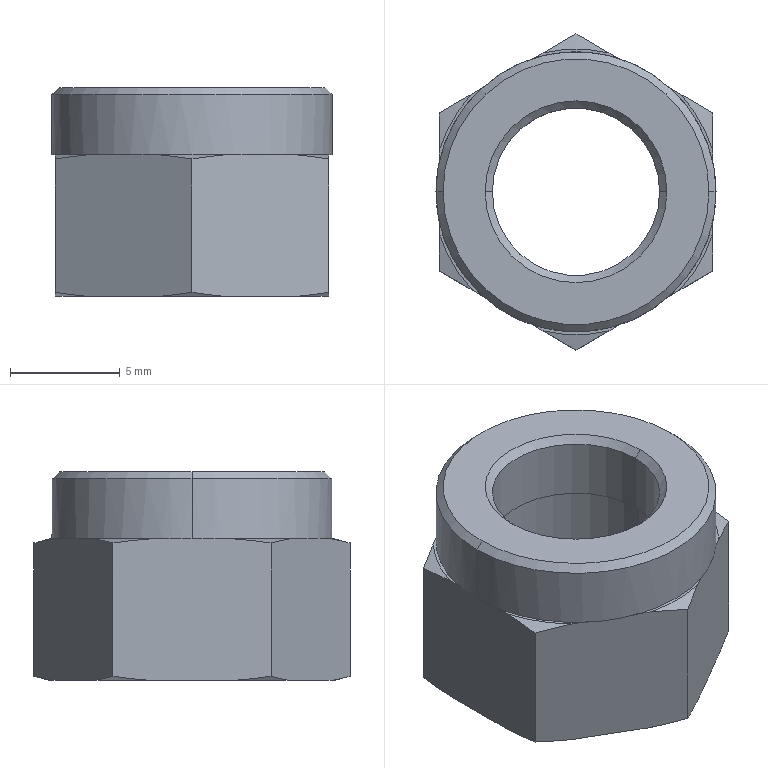Part | SolidWorks | features Cut 3, Boss 1, Chamfer 1, Extrusion 1 | 1 solid | 43 faces | box 12.74 x 14.38 x 9.5 mm | volume 787.765 mm3 | plane 21 | cone 16 | cylinder 6 | commonest cylinder face diameters 7.619 x2 8 x2 12.74 x2
STEP:
#1=CARTESIAN_POINT('',(-3.81,0.,9.175));
#2=VERTEX_POINT('',#1);
#3=CARTESIAN_POINT('',(3.81,0.,9.175));
#4=VERTEX_POINT('',#3);
#5=CARTESIAN_POINT('',(0.,0.,9.175));
#6=DIRECTION('',(0.,0.,1.));
#7=DIRECTION('',(1.,0.,0.));
#8=AXIS2_PLACEMENT_3D('',#5,#6,#7);
#9=CIRCLE('',#8,3.81);
#10=EDGE_CURVE('',#2,#4,#9,.T.);
#11=ORIENTED_EDGE('',*,*,#10,.F.);
#12=CARTESIAN_POINT('',(-4.135,0.,9.5));
#13=VERTEX_POINT('',#12);
#14=CARTESIAN_POINT('',(-3.81,0.,9.175));
#15=DIRECTION('',(-0.7071,0.,0.7071));
#16=VECTOR('',#15,1000.);
#17=LINE('',#14,#16);
#18=EDGE_CURVE('',#2,#13,#17,.T.);
#19=ORIENTED_EDGE('',*,*,#18,.T.);
#20=CARTESIAN_POINT('',(4.135,0.,9.5));
#21=VERTEX_POINT('',#20);
#22=CARTESIAN_POINT('',(0.,0.,9.5));
#23=DIRECTION('',(0.,0.,-1.));
#24=DIRECTION('',(1.,0.,0.));
#25=AXIS2_PLACEMENT_3D('',#22,#23,#24);
#26=CIRCLE('',#25,4.135);
#27=EDGE_CURVE('',#21,#13,#26,.T.);
#28=ORIENTED_EDGE('',*,*,#27,.F.);
#29=CARTESIAN_POINT('',(3.81,0.,9.175));
#30=DIRECTION('',(0.7071,0.,0.7071));
#31=VECTOR('',#30,1000.);
#32=LINE('',#29,#31);
#33=EDGE_CURVE('',#4,#21,#32,.T.);
#34=ORIENTED_EDGE('',*,*,#33,.F.);
#35=EDGE_LOOP('',(#11,#19,#28,#34));
#36=FACE_OUTER_BOUND('',#35,.T.);
#37=CARTESIAN_POINT('',(0.,0.,9.175));
#38=DIRECTION('',(0.,0.,1.));
#39=DIRECTION('',(1.,0.,0.));
#40=AXIS2_PLACEMENT_3D('',#37,#38,#39);
#41=CONICAL_SURFACE('',#40,3.81,0.7854);
#42=ADVANCED_FACE('',(#36),#41,.F.);
#43=CARTESIAN_POINT('',(6.045,0.,9.5));
#44=VERTEX_POINT('',#43);
#45=CARTESIAN_POINT('',(-6.045,0.,9.5));
#46=VERTEX_POINT('',#45);
#47=CARTESIAN_POINT('',(0.,0.,9.5));
#48=DIRECTION('',(0.,0.,1.));
#49=DIRECTION('',(1.,0.,0.));
#50=AXIS2_PLACEMENT_3D('',#47,#48,#49);
#51=CIRCLE('',#50,6.045);
#52=EDGE_CURVE('',#44,#46,#51,.T.);
#53=ORIENTED_EDGE('',*,*,#52,.F.);
#54=CARTESIAN_POINT('',(6.37,0.,9.175));
#55=VERTEX_POINT('',#54);
#56=CARTESIAN_POINT('',(6.045,0.,9.5));
#57=DIRECTION('',(0.7071,0.,-0.7071));
#58=VECTOR('',#57,1000.);
#59=LINE('',#56,#58);
#60=EDGE_CURVE('',#44,#55,#59,.T.);
#61=ORIENTED_EDGE('',*,*,#60,.T.);
#62=CARTESIAN_POINT('',(-6.37,0.,9.175));
#63=VERTEX_POINT('',#62);
#64=CARTESIAN_POINT('',(0.,0.,9.175));
#65=DIRECTION('',(0.,0.,-1.));
#66=DIRECTION('',(1.,0.,0.));
#67=AXIS2_PLACEMENT_3D('',#64,#65,#66);
#68=CIRCLE('',#67,6.37);
#69=EDGE_CURVE('',#63,#55,#68,.T.);
#70=ORIENTED_EDGE('',*,*,#69,.F.);
#71=CARTESIAN_POINT('',(-6.045,0.,9.5));
#72=DIRECTION('',(-0.7071,0.,-0.7071));
#73=VECTOR('',#72,1000.);
#74=LINE('',#71,#73);
#75=EDGE_CURVE('',#46,#63,#74,.T.);
#76=ORIENTED_EDGE('',*,*,#75,.F.);
#77=EDGE_LOOP('',(#53,#61,#70,#76));
#78=FACE_OUTER_BOUND('',#77,.T.);
#79=CARTESIAN_POINT('',(0.,0.,9.5));
#80=DIRECTION('',(0.,0.,-1.));
#81=DIRECTION('',(-1.,0.,0.));
#82=AXIS2_PLACEMENT_3D('',#79,#80,#81);
#83=CONICAL_SURFACE('',#82,6.045,0.7854);
#84=ADVANCED_FACE('',(#78),#83,.T.);
#85=CARTESIAN_POINT('',(-3.81,0.,6.44));
#86=VERTEX_POINT('',#85);
#87=CARTESIAN_POINT('',(3.81,0.,6.44));
#88=VERTEX_POINT('',#87);
#89=CARTESIAN_POINT('',(0.,0.,6.44));
#90=DIRECTION('',(0.,0.,1.));
#91=DIRECTION('',(1.,0.,0.));
#92=AXIS2_PLACEMENT_3D('',#89,#90,#91);
#93=CIRCLE('',#92,3.81);
#94=EDGE_CURVE('',#86,#88,#93,.T.);
#95=ORIENTED_EDGE('',*,*,#94,.F.);
#96=CARTESIAN_POINT('',(-3.81,0.,0.));
#97=DIRECTION('',(0.,0.,1.));
#98=VECTOR('',#97,1000.);
#99=LINE('',#96,#98);
#100=EDGE_CURVE('',#86,#2,#99,.T.);
#101=ORIENTED_EDGE('',*,*,#100,.T.);
#102=ORIENTED_EDGE('',*,*,#10,.T.);
#103=CARTESIAN_POINT('',(3.81,0.,0.));
#104=DIRECTION('',(0.,0.,1.));
#105=VECTOR('',#104,1000.);
#106=LINE('',#103,#105);
#107=EDGE_CURVE('',#88,#4,#106,.T.);
#108=ORIENTED_EDGE('',*,*,#107,.F.);
#109=EDGE_LOOP('',(#95,#101,#102,#108));
#110=FACE_OUTER_BOUND('',#109,.T.);
#111=CARTESIAN_POINT('',(0.,0.,0.));
#112=DIRECTION('',(0.,0.,1.));
#113=DIRECTION('',(1.,0.,0.));
#114=AXIS2_PLACEMENT_3D('',#111,#112,#113);
#115=CYLINDRICAL_SURFACE('',#114,3.81);
#116=ADVANCED_FACE('',(#110),#115,.F.);
#117=ORIENTED_EDGE('',*,*,#69,.T.);
#118=CARTESIAN_POINT('',(6.37,0.,6.44));
#119=VERTEX_POINT('',#118);
#120=CARTESIAN_POINT('',(6.37,0.,9.5));
#121=DIRECTION('',(0.,0.,-1.));
#122=VECTOR('',#121,1000.);
#123=LINE('',#120,#122);
#124=EDGE_CURVE('',#55,#119,#123,.T.);
#125=ORIENTED_EDGE('',*,*,#124,.T.);
#126=CARTESIAN_POINT('',(6.227,1.343,6.44));
#127=VERTEX_POINT('',#126);
#128=CARTESIAN_POINT('',(0.,0.,6.44));
#129=DIRECTION('',(0.,0.,1.));
#130=DIRECTION('',(1.,0.,0.));
#131=AXIS2_PLACEMENT_3D('',#128,#129,#130);
#132=CIRCLE('',#131,6.37);
#133=EDGE_CURVE('',#119,#127,#132,.T.);
#134=ORIENTED_EDGE('',*,*,#133,.T.);
#135=CARTESIAN_POINT('',(4.277,4.721,6.44));
#136=VERTEX_POINT('',#135);
#137=CARTESIAN_POINT('',(0.,0.,6.44));
#138=DIRECTION('',(0.,0.,1.));
#139=DIRECTION('',(1.,0.,0.));
#140=AXIS2_PLACEMENT_3D('',#137,#138,#139);
#141=CIRCLE('',#140,6.37);
#142=EDGE_CURVE('',#127,#136,#141,.T.);
#143=ORIENTED_EDGE('',*,*,#142,.T.);
#144=CARTESIAN_POINT('',(1.95,6.064,6.44));
#145=VERTEX_POINT('',#144);
#146=CARTESIAN_POINT('',(0.,0.,6.44));
#147=DIRECTION('',(0.,0.,1.));
#148=DIRECTION('',(1.,0.,0.));
#149=AXIS2_PLACEMENT_3D('',#146,#147,#148);
#150=CIRCLE('',#149,6.37);
#151=EDGE_CURVE('',#136,#145,#150,.T.);
#152=ORIENTED_EDGE('',*,*,#151,.T.);
#153=CARTESIAN_POINT('',(-1.95,6.064,6.44));
#154=VERTEX_POINT('',#153);
#155=CARTESIAN_POINT('',(0.,0.,6.44));
#156=DIRECTION('',(0.,0.,1.));
#157=DIRECTION('',(1.,0.,0.));
#158=AXIS2_PLACEMENT_3D('',#155,#156,#157);
#159=CIRCLE('',#158,6.37);
#160=EDGE_CURVE('',#145,#154,#159,.T.);
#161=ORIENTED_EDGE('',*,*,#160,.T.);
#162=CARTESIAN_POINT('',(-4.277,4.721,6.44));
#163=VERTEX_POINT('',#162);
#164=CARTESIAN_POINT('',(0.,0.,6.44));
#165=DIRECTION('',(0.,0.,1.));
#166=DIRECTION('',(1.,0.,0.));
#167=AXIS2_PLACEMENT_3D('',#164,#165,#166);
#168=CIRCLE('',#167,6.37);
#169=EDGE_CURVE('',#154,#163,#168,.T.);
#170=ORIENTED_EDGE('',*,*,#169,.T.);
#171=CARTESIAN_POINT('',(-6.227,1.343,6.44));
#172=VERTEX_POINT('',#171);
#173=CARTESIAN_POINT('',(0.,0.,6.44));
#174=DIRECTION('',(0.,0.,1.));
#175=DIRECTION('',(1.,0.,0.));
#176=AXIS2_PLACEMENT_3D('',#173,#174,#175);
#177=CIRCLE('',#176,6.37);
#178=EDGE_CURVE('',#163,#172,#177,.T.);
#179=ORIENTED_EDGE('',*,*,#178,.T.);
#180=CARTESIAN_POINT('',(-6.37,0.,6.44));
#181=VERTEX_POINT('',#180);
#182=CARTESIAN_POINT('',(0.,0.,6.44));
#183=DIRECTION('',(0.,0.,1.));
#184=DIRECTION('',(1.,0.,0.));
#185=AXIS2_PLACEMENT_3D('',#182,#183,#184);
#186=CIRCLE('',#185,6.37);
#187=EDGE_CURVE('',#172,#181,#186,.T.);
#188=ORIENTED_EDGE('',*,*,#187,.T.);
#189=CARTESIAN_POINT('',(-6.37,0.,9.5));
#190=DIRECTION('',(0.,0.,-1.));
#191=VECTOR('',#190,1000.);
#192=LINE('',#189,#191);
#193=EDGE_CURVE('',#63,#181,#192,.T.);
#194=ORIENTED_EDGE('',*,*,#193,.F.);
#195=EDGE_LOOP('',(#117,#125,#134,#143,#152,#161,#170,#179,#188,#194));
#196=FACE_OUTER_BOUND('',#195,.T.);
#197=CARTESIAN_POINT('',(0.,0.,9.5));
#198=DIRECTION('',(0.,0.,-1.));
#199=DIRECTION('',(-1.,0.,0.));
#200=AXIS2_PLACEMENT_3D('',#197,#198,#199);
#201=CYLINDRICAL_SURFACE('',#200,6.37);
#202=ADVANCED_FACE('',(#196),#201,.T.);
#203=CARTESIAN_POINT('',(-4.,0.,6.44));
#204=VERTEX_POINT('',#203);
#205=CARTESIAN_POINT('',(4.,0.,6.44));
#206=VERTEX_POINT('',#205);
#207=CARTESIAN_POINT('',(0.,0.,6.44));
#208=DIRECTION('',(0.,0.,1.));
#209=DIRECTION('',(1.,0.,0.));
#210=AXIS2_PLACEMENT_3D('',#207,#208,#209);
#211=CIRCLE('',#210,4.);
#212=EDGE_CURVE('',#204,#206,#211,.T.);
#213=ORIENTED_EDGE('',*,*,#212,.T.);
#214=CARTESIAN_POINT('',(4.,0.,0.));
#215=VERTEX_POINT('',#214);
#216=CARTESIAN_POINT('',(4.,0.,6.44));
#217=DIRECTION('',(0.,0.,-1.));
#218=VECTOR('',#217,1000.);
#219=LINE('',#216,#218);
#220=EDGE_CURVE('',#206,#215,#219,.T.);
#221=ORIENTED_EDGE('',*,*,#220,.T.);
#222=CARTESIAN_POINT('',(-4.,0.,0.));
#223=VERTEX_POINT('',#222);
#224=CARTESIAN_POINT('',(0.,0.,0.));
#225=DIRECTION('',(0.,0.,1.));
#226=DIRECTION('',(1.,0.,0.));
#227=AXIS2_PLACEMENT_3D('',#224,#225,#226);
#228=CIRCLE('',#227,4.);
#229=EDGE_CURVE('',#223,#215,#228,.T.);
#230=ORIENTED_EDGE('',*,*,#229,.F.);
#231=CARTESIAN_POINT('',(-4.,0.,6.44));
#232=DIRECTION('',(0.,0.,-1.));
#233=VECTOR('',#232,1000.);
#234=LINE('',#231,#233);
#235=EDGE_CURVE('',#204,#223,#234,.T.);
#236=ORIENTED_EDGE('',*,*,#235,.F.);
#237=EDGE_LOOP('',(#213,#221,#230,#236));
#238=FACE_OUTER_BOUND('',#237,.T.);
#239=CARTESIAN_POINT('',(0.,0.,6.44));
#240=DIRECTION('',(0.,0.,-1.));
#241=DIRECTION('',(-1.,0.,0.));
#242=AXIS2_PLACEMENT_3D('',#239,#240,#241);
#243=CYLINDRICAL_SURFACE('',#242,4.);
#244=ADVANCED_FACE('',(#238),#243,.F.);
#245=CARTESIAN_POINT('',(-6.227,-1.343,6.44));
#246=VERTEX_POINT('',#245);
#247=CARTESIAN_POINT('',(-4.277,-4.721,6.44));
#248=VERTEX_POINT('',#247);
#249=CARTESIAN_POINT('',(0.,0.,6.44));
#250=DIRECTION('',(0.,0.,1.));
#251=DIRECTION('',(1.,0.,0.));
#252=AXIS2_PLACEMENT_3D('',#249,#250,#251);
#253=CIRCLE('',#252,6.37);
#254=EDGE_CURVE('',#246,#248,#253,.T.);
#255=ORIENTED_EDGE('',*,*,#254,.F.);
#256=CARTESIAN_POINT('',(-6.227,-1.865,6.44));
#257=VERTEX_POINT('',#256);
#258=CARTESIAN_POINT('',(-6.227,3.595,6.44));
#259=DIRECTION('',(0.,-1.,0.));
#260=VECTOR('',#259,1000.);
#261=LINE('',#258,#260);
#262=EDGE_CURVE('',#246,#257,#261,.T.);
#263=ORIENTED_EDGE('',*,*,#262,.T.);
#264=CARTESIAN_POINT('',(-4.728,-4.46,6.44));
#265=VERTEX_POINT('',#264);
#266=CARTESIAN_POINT('',(0.,0.,6.44));
#267=DIRECTION('',(0.,0.,1.));
#268=DIRECTION('',(1.,0.,0.));
#269=AXIS2_PLACEMENT_3D('',#266,#267,#268);
#270=CIRCLE('',#269,6.5);
#271=EDGE_CURVE('',#257,#265,#270,.T.);
#272=ORIENTED_EDGE('',*,*,#271,.T.);
#273=CARTESIAN_POINT('',(-6.227,-3.595,6.44));
#274=DIRECTION('',(0.866,-0.5,0.));
#275=VECTOR('',#274,1000.);
#276=LINE('',#273,#275);
#277=EDGE_CURVE('',#265,#248,#276,.T.);
#278=ORIENTED_EDGE('',*,*,#277,.T.);
#279=EDGE_LOOP('',(#255,#263,#272,#278));
#280=FACE_OUTER_BOUND('',#279,.T.);
#281=CARTESIAN_POINT('',(6.227,3.595,6.44));
#282=DIRECTION('',(0.,0.,-1.));
#283=DIRECTION('',(-1.,0.,0.));
#284=AXIS2_PLACEMENT_3D('',#281,#282,#283);
#285=PLANE('',#284);
#286=ADVANCED_FACE('',(#280),#285,.F.);
#287=CARTESIAN_POINT('',(-1.95,-6.064,6.44));
#288=VERTEX_POINT('',#287);
#289=CARTESIAN_POINT('',(1.95,-6.064,6.44));
#290=VERTEX_POINT('',#289);
#291=CARTESIAN_POINT('',(0.,0.,6.44));
#292=DIRECTION('',(0.,0.,1.));
#293=DIRECTION('',(1.,0.,0.));
#294=AXIS2_PLACEMENT_3D('',#291,#292,#293);
#295=CIRCLE('',#294,6.37);
#296=EDGE_CURVE('',#288,#290,#295,.T.);
#297=ORIENTED_EDGE('',*,*,#296,.F.);
#298=CARTESIAN_POINT('',(-1.498,-6.325,6.44));
#299=VERTEX_POINT('',#298);
#300=CARTESIAN_POINT('',(-6.227,-3.595,6.44));
#301=DIRECTION('',(0.866,-0.5,0.));
#302=VECTOR('',#301,1000.);
#303=LINE('',#300,#302);
#304=EDGE_CURVE('',#288,#299,#303,.T.);
#305=ORIENTED_EDGE('',*,*,#304,.T.);
#306=CARTESIAN_POINT('',(1.498,-6.325,6.44));
#307=VERTEX_POINT('',#306);
#308=CARTESIAN_POINT('',(0.,0.,6.44));
#309=DIRECTION('',(0.,0.,1.));
#310=DIRECTION('',(1.,0.,0.));
#311=AXIS2_PLACEMENT_3D('',#308,#309,#310);
#312=CIRCLE('',#311,6.5);
#313=EDGE_CURVE('',#299,#307,#312,.T.);
#314=ORIENTED_EDGE('',*,*,#313,.T.);
#315=CARTESIAN_POINT('',(0.,-7.19,6.44));
#316=DIRECTION('',(0.866,0.5,0.));
#317=VECTOR('',#316,1000.);
#318=LINE('',#315,#317);
#319=EDGE_CURVE('',#307,#290,#318,.T.);
#320=ORIENTED_EDGE('',*,*,#319,.T.);
#321=EDGE_LOOP('',(#297,#305,#314,#320));
#322=FACE_OUTER_BOUND('',#321,.T.);
#323=CARTESIAN_POINT('',(6.227,3.595,6.44));
#324=DIRECTION('',(0.,0.,-1.));
#325=DIRECTION('',(-1.,0.,0.));
#326=AXIS2_PLACEMENT_3D('',#323,#324,#325);
#327=PLANE('',#326);
#328=ADVANCED_FACE('',(#322),#327,.F.);
#329=CARTESIAN_POINT('',(4.277,-4.721,6.44));
#330=VERTEX_POINT('',#329);
#331=CARTESIAN_POINT('',(6.227,-1.343,6.44));
#332=VERTEX_POINT('',#331);
#333=CARTESIAN_POINT('',(0.,0.,6.44));
#334=DIRECTION('',(0.,0.,1.));
#335=DIRECTION('',(1.,0.,0.));
#336=AXIS2_PLACEMENT_3D('',#333,#334,#335);
#337=CIRCLE('',#336,6.37);
#338=EDGE_CURVE('',#330,#332,#337,.T.);
#339=ORIENTED_EDGE('',*,*,#338,.F.);
#340=CARTESIAN_POINT('',(4.728,-4.46,6.44));
#341=VERTEX_POINT('',#340);
#342=CARTESIAN_POINT('',(0.,-7.19,6.44));
#343=DIRECTION('',(0.866,0.5,0.));
#344=VECTOR('',#343,1000.);
#345=LINE('',#342,#344);
#346=EDGE_CURVE('',#330,#341,#345,.T.);
#347=ORIENTED_EDGE('',*,*,#346,.T.);
#348=CARTESIAN_POINT('',(6.227,-1.865,6.44));
#349=VERTEX_POINT('',#348);
#350=CARTESIAN_POINT('',(0.,0.,6.44));
#351=DIRECTION('',(0.,0.,1.));
#352=DIRECTION('',(1.,0.,0.));
#353=AXIS2_PLACEMENT_3D('',#350,#351,#352);
#354=CIRCLE('',#353,6.5);
#355=EDGE_CURVE('',#341,#349,#354,.T.);
#356=ORIENTED_EDGE('',*,*,#355,.T.);
#357=CARTESIAN_POINT('',(6.227,-3.595,6.44));
#358=DIRECTION('',(0.,1.,0.));
#359=VECTOR('',#358,1000.);
#360=LINE('',#357,#359);
#361=EDGE_CURVE('',#349,#332,#360,.T.);
#362=ORIENTED_EDGE('',*,*,#361,.T.);
#363=EDGE_LOOP('',(#339,#347,#356,#362));
#364=FACE_OUTER_BOUND('',#363,.T.);
#365=CARTESIAN_POINT('',(6.227,3.595,6.44));
#366=DIRECTION('',(0.,0.,-1.));
#367=DIRECTION('',(-1.,0.,0.));
#368=AXIS2_PLACEMENT_3D('',#365,#366,#367);
#369=PLANE('',#368);
#370=ADVANCED_FACE('',(#364),#369,.F.);
#371=ORIENTED_EDGE('',*,*,#142,.F.);
#372=CARTESIAN_POINT('',(6.227,1.865,6.44));
#373=VERTEX_POINT('',#372);
#374=CARTESIAN_POINT('',(6.227,-3.595,6.44));
#375=DIRECTION('',(0.,1.,0.));
#376=VECTOR('',#375,1000.);
#377=LINE('',#374,#376);
#378=EDGE_CURVE('',#127,#373,#377,.T.);
#379=ORIENTED_EDGE('',*,*,#378,.T.);
#380=CARTESIAN_POINT('',(4.728,4.46,6.44));
#381=VERTEX_POINT('',#380);
#382=CARTESIAN_POINT('',(0.,0.,6.44));
#383=DIRECTION('',(0.,0.,1.));
#384=DIRECTION('',(1.,0.,0.));
#385=AXIS2_PLACEMENT_3D('',#382,#383,#384);
#386=CIRCLE('',#385,6.5);
#387=EDGE_CURVE('',#373,#381,#386,.T.);
#388=ORIENTED_EDGE('',*,*,#387,.T.);
#389=CARTESIAN_POINT('',(6.227,3.595,6.44));
#390=DIRECTION('',(-0.866,0.5,0.));
#391=VECTOR('',#390,1000.);
#392=LINE('',#389,#391);
#393=EDGE_CURVE('',#381,#136,#392,.T.);
#394=ORIENTED_EDGE('',*,*,#393,.T.);
#395=EDGE_LOOP('',(#371,#379,#388,#394));
#396=FACE_OUTER_BOUND('',#395,.T.);
#397=CARTESIAN_POINT('',(6.227,3.595,6.44));
#398=DIRECTION('',(0.,0.,-1.));
#399=DIRECTION('',(-1.,0.,0.));
#400=AXIS2_PLACEMENT_3D('',#397,#398,#399);
#401=PLANE('',#400);
#402=ADVANCED_FACE('',(#396),#401,.F.);
#403=ORIENTED_EDGE('',*,*,#160,.F.);
#404=CARTESIAN_POINT('',(1.498,6.325,6.44));
#405=VERTEX_POINT('',#404);
#406=CARTESIAN_POINT('',(6.227,3.595,6.44));
#407=DIRECTION('',(-0.866,0.5,0.));
#408=VECTOR('',#407,1000.);
#409=LINE('',#406,#408);
#410=EDGE_CURVE('',#145,#405,#409,.T.);
#411=ORIENTED_EDGE('',*,*,#410,.T.);
#412=CARTESIAN_POINT('',(-1.498,6.325,6.44));
#413=VERTEX_POINT('',#412);
#414=CARTESIAN_POINT('',(0.,0.,6.44));
#415=DIRECTION('',(0.,0.,1.));
#416=DIRECTION('',(1.,0.,0.));
#417=AXIS2_PLACEMENT_3D('',#414,#415,#416);
#418=CIRCLE('',#417,6.5);
#419=EDGE_CURVE('',#405,#413,#418,.T.);
#420=ORIENTED_EDGE('',*,*,#419,.T.);
#421=CARTESIAN_POINT('',(0.,7.19,6.44));
#422=DIRECTION('',(-0.866,-0.5,0.));
#423=VECTOR('',#422,1000.);
#424=LINE('',#421,#423);
#425=EDGE_CURVE('',#413,#154,#424,.T.);
#426=ORIENTED_EDGE('',*,*,#425,.T.);
#427=EDGE_LOOP('',(#403,#411,#420,#426));
#428=FACE_OUTER_BOUND('',#427,.T.);
#429=CARTESIAN_POINT('',(6.227,3.595,6.44));
#430=DIRECTION('',(0.,0.,-1.));
#431=DIRECTION('',(-1.,0.,0.));
#432=AXIS2_PLACEMENT_3D('',#429,#430,#431);
#433=PLANE('',#432);
#434=ADVANCED_FACE('',(#428),#433,.F.);
#435=ORIENTED_EDGE('',*,*,#178,.F.);
#436=CARTESIAN_POINT('',(-4.728,4.46,6.44));
#437=VERTEX_POINT('',#436);
#438=CARTESIAN_POINT('',(0.,7.19,6.44));
#439=DIRECTION('',(-0.866,-0.5,0.));
#440=VECTOR('',#439,1000.);
#441=LINE('',#438,#440);
#442=EDGE_CURVE('',#163,#437,#441,.T.);
#443=ORIENTED_EDGE('',*,*,#442,.T.);
#444=CARTESIAN_POINT('',(-6.227,1.865,6.44));
#445=VERTEX_POINT('',#444);
#446=CARTESIAN_POINT('',(0.,0.,6.44));
#447=DIRECTION('',(0.,0.,1.));
#448=DIRECTION('',(1.,0.,0.));
#449=AXIS2_PLACEMENT_3D('',#446,#447,#448);
#450=CIRCLE('',#449,6.5);
#451=EDGE_CURVE('',#437,#445,#450,.T.);
#452=ORIENTED_EDGE('',*,*,#451,.T.);
#453=CARTESIAN_POINT('',(-6.227,3.595,6.44));
#454=DIRECTION('',(0.,-1.,0.));
#455=VECTOR('',#454,1000.);
#456=LINE('',#453,#455);
#457=EDGE_CURVE('',#445,#172,#456,.T.);
#458=ORIENTED_EDGE('',*,*,#457,.T.);
#459=EDGE_LOOP('',(#435,#443,#452,#458));
#460=FACE_OUTER_BOUND('',#459,.T.);
#461=CARTESIAN_POINT('',(6.227,3.595,6.44));
#462=DIRECTION('',(0.,0.,-1.));
#463=DIRECTION('',(-1.,0.,0.));
#464=AXIS2_PLACEMENT_3D('',#461,#462,#463);
#465=PLANE('',#464);
#466=ADVANCED_FACE('',(#460),#465,.F.);
#467=CARTESIAN_POINT('',(0.,7.19,0.1849));
#468=VERTEX_POINT('',#467);
#469=CARTESIAN_POINT('',(1.498,6.325,0.));
#470=VERTEX_POINT('',#469);
#471=CARTESIAN_POINT('',(0.,7.19,0.1849));
#472=CARTESIAN_POINT('',(0.4978,6.903,0.1079));
#473=CARTESIAN_POINT('',(0.9971,6.614,0.04449));
#474=CARTESIAN_POINT('',(1.498,6.325,0.));
#475=B_SPLINE_CURVE_WITH_KNOTS('',3,(#471,#472,#473,#474),.UNSPECIFIED.,.F.,.F.,(4,4),(0.006757,0.008497),.UNSPECIFIED.);
#476=EDGE_CURVE('',#468,#470,#475,.T.);
#477=ORIENTED_EDGE('',*,*,#476,.F.);
#478=CARTESIAN_POINT('',(0.,7.19,6.255));
#479=VERTEX_POINT('',#478);
#480=CARTESIAN_POINT('',(0.,7.19,6.44));
#481=DIRECTION('',(0.,0.,-1.));
#482=VECTOR('',#481,1000.);
#483=LINE('',#480,#482);
#484=EDGE_CURVE('',#479,#468,#483,.T.);
#485=ORIENTED_EDGE('',*,*,#484,.F.);
#486=CARTESIAN_POINT('',(1.498,6.325,6.44));
#487=CARTESIAN_POINT('',(0.9966,6.615,6.395));
#488=CARTESIAN_POINT('',(0.4971,6.903,6.332));
#489=CARTESIAN_POINT('',(0.,7.19,6.255));
#490=B_SPLINE_CURVE_WITH_KNOTS('',3,(#486,#487,#488,#489),.UNSPECIFIED.,.F.,.F.,(4,4),(0.0122,0.01391),.UNSPECIFIED.);
#491=EDGE_CURVE('',#405,#479,#490,.T.);
#492=ORIENTED_EDGE('',*,*,#491,.F.);
#493=ORIENTED_EDGE('',*,*,#410,.F.);
#494=CARTESIAN_POINT('',(6.227,3.595,6.44));
#495=DIRECTION('',(-0.866,0.5,0.));
#496=VECTOR('',#495,1000.);
#497=LINE('',#494,#496);
#498=EDGE_CURVE('',#136,#145,#497,.T.);
#499=ORIENTED_EDGE('',*,*,#498,.F.);
#500=ORIENTED_EDGE('',*,*,#393,.F.);
#501=CARTESIAN_POINT('',(6.227,3.595,6.255));
#502=VERTEX_POINT('',#501);
#503=CARTESIAN_POINT('',(6.227,3.595,6.255));
#504=CARTESIAN_POINT('',(5.729,3.882,6.332));
#505=CARTESIAN_POINT('',(5.23,4.171,6.396));
#506=CARTESIAN_POINT('',(4.728,4.46,6.44));
#507=B_SPLINE_CURVE_WITH_KNOTS('',3,(#503,#504,#505,#506),.UNSPECIFIED.,.F.,.F.,(4,4),(0.006757,0.008497),.UNSPECIFIED.);
#508=EDGE_CURVE('',#502,#381,#507,.T.);
#509=ORIENTED_EDGE('',*,*,#508,.F.);
#510=CARTESIAN_POINT('',(6.227,3.595,0.1849));
#511=VERTEX_POINT('',#510);
#512=CARTESIAN_POINT('',(6.227,3.595,6.44));
#513=DIRECTION('',(0.,0.,-1.));
#514=VECTOR('',#513,1000.);
#515=LINE('',#512,#514);
#516=EDGE_CURVE('',#502,#511,#515,.T.);
#517=ORIENTED_EDGE('',*,*,#516,.T.);
#518=CARTESIAN_POINT('',(4.728,4.46,0.));
#519=VERTEX_POINT('',#518);
#520=CARTESIAN_POINT('',(4.728,4.46,0.));
#521=CARTESIAN_POINT('',(5.23,4.17,0.04453));
#522=CARTESIAN_POINT('',(5.73,3.882,0.108));
#523=CARTESIAN_POINT('',(6.227,3.595,0.1849));
#524=B_SPLINE_CURVE_WITH_KNOTS('',3,(#520,#521,#522,#523),.UNSPECIFIED.,.F.,.F.,(4,4),(0.0122,0.01391),.UNSPECIFIED.);
#525=EDGE_CURVE('',#519,#511,#524,.T.);
#526=ORIENTED_EDGE('',*,*,#525,.F.);
#527=CARTESIAN_POINT('',(6.227,3.595,0.));
#528=DIRECTION('',(-0.866,0.5,0.));
#529=VECTOR('',#528,1000.);
#530=LINE('',#527,#529);
#531=EDGE_CURVE('',#519,#470,#530,.T.);
#532=ORIENTED_EDGE('',*,*,#531,.T.);
#533=EDGE_LOOP('',(#477,#485,#492,#493,#499,#500,#509,#517,#526,#532));
#534=FACE_OUTER_BOUND('',#533,.T.);
#535=CARTESIAN_POINT('',(6.227,3.595,6.44));
#536=DIRECTION('',(-0.5,-0.866,0.));
#537=DIRECTION('',(0.866,-0.5,0.));
#538=AXIS2_PLACEMENT_3D('',#535,#536,#537);
#539=PLANE('',#538);
#540=ADVANCED_FACE('',(#534),#539,.F.);
#541=CARTESIAN_POINT('',(-6.227,3.595,0.1849));
#542=VERTEX_POINT('',#541);
#543=CARTESIAN_POINT('',(-4.728,4.46,0.));
#544=VERTEX_POINT('',#543);
#545=CARTESIAN_POINT('',(-6.227,3.595,0.1849));
#546=CARTESIAN_POINT('',(-5.729,3.882,0.1079));
#547=CARTESIAN_POINT('',(-5.23,4.171,0.04449));
#548=CARTESIAN_POINT('',(-4.728,4.46,0.));
#549=B_SPLINE_CURVE_WITH_KNOTS('',3,(#545,#546,#547,#548),.UNSPECIFIED.,.F.,.F.,(4,4),(0.006757,0.008497),.UNSPECIFIED.);
#550=EDGE_CURVE('',#542,#544,#549,.T.);
#551=ORIENTED_EDGE('',*,*,#550,.F.);
#552=CARTESIAN_POINT('',(-6.227,3.595,6.255));
#553=VERTEX_POINT('',#552);
#554=CARTESIAN_POINT('',(-6.227,3.595,6.44));
#555=DIRECTION('',(0.,0.,-1.));
#556=VECTOR('',#555,1000.);
#557=LINE('',#554,#556);
#558=EDGE_CURVE('',#553,#542,#557,.T.);
#559=ORIENTED_EDGE('',*,*,#558,.F.);
#560=CARTESIAN_POINT('',(-4.728,4.46,6.44));
#561=CARTESIAN_POINT('',(-5.23,4.17,6.395));
#562=CARTESIAN_POINT('',(-5.73,3.882,6.332));
#563=CARTESIAN_POINT('',(-6.227,3.595,6.255));
#564=B_SPLINE_CURVE_WITH_KNOTS('',3,(#560,#561,#562,#563),.UNSPECIFIED.,.F.,.F.,(4,4),(0.0122,0.01391),.UNSPECIFIED.);
#565=EDGE_CURVE('',#437,#553,#564,.T.);
#566=ORIENTED_EDGE('',*,*,#565,.F.);
#567=ORIENTED_EDGE('',*,*,#442,.F.);
#568=CARTESIAN_POINT('',(0.,7.19,6.44));
#569=DIRECTION('',(-0.866,-0.5,0.));
#570=VECTOR('',#569,1000.);
#571=LINE('',#568,#570);
#572=EDGE_CURVE('',#154,#163,#571,.T.);
#573=ORIENTED_EDGE('',*,*,#572,.F.);
#574=ORIENTED_EDGE('',*,*,#425,.F.);
#575=CARTESIAN_POINT('',(0.,7.19,6.255));
#576=CARTESIAN_POINT('',(-0.4978,6.903,6.332));
#577=CARTESIAN_POINT('',(-0.9971,6.614,6.396));
#578=CARTESIAN_POINT('',(-1.498,6.325,6.44));
#579=B_SPLINE_CURVE_WITH_KNOTS('',3,(#575,#576,#577,#578),.UNSPECIFIED.,.F.,.F.,(4,4),(0.006757,0.008497),.UNSPECIFIED.);
#580=EDGE_CURVE('',#479,#413,#579,.T.);
#581=ORIENTED_EDGE('',*,*,#580,.F.);
#582=ORIENTED_EDGE('',*,*,#484,.T.);
#583=CARTESIAN_POINT('',(-1.498,6.325,0.));
#584=VERTEX_POINT('',#583);
#585=CARTESIAN_POINT('',(-1.498,6.325,0.));
#586=CARTESIAN_POINT('',(-0.9966,6.615,0.04453));
#587=CARTESIAN_POINT('',(-0.4971,6.903,0.108));
#588=CARTESIAN_POINT('',(0.,7.19,0.1849));
#589=B_SPLINE_CURVE_WITH_KNOTS('',3,(#585,#586,#587,#588),.UNSPECIFIED.,.F.,.F.,(4,4),(0.0122,0.01391),.UNSPECIFIED.);
#590=EDGE_CURVE('',#584,#468,#589,.T.);
#591=ORIENTED_EDGE('',*,*,#590,.F.);
#592=CARTESIAN_POINT('',(0.,7.19,0.));
#593=DIRECTION('',(-0.866,-0.5,0.));
#594=VECTOR('',#593,1000.);
#595=LINE('',#592,#594);
#596=EDGE_CURVE('',#584,#544,#595,.T.);
#597=ORIENTED_EDGE('',*,*,#596,.T.);
#598=EDGE_LOOP('',(#551,#559,#566,#567,#573,#574,#581,#582,#591,#597));
#599=FACE_OUTER_BOUND('',#598,.T.);
#600=CARTESIAN_POINT('',(0.,7.19,6.44));
#601=DIRECTION('',(0.5,-0.866,0.));
#602=DIRECTION('',(0.866,0.5,0.));
#603=AXIS2_PLACEMENT_3D('',#600,#601,#602);
#604=PLANE('',#603);
#605=ADVANCED_FACE('',(#599),#604,.F.);
#606=CARTESIAN_POINT('',(-6.227,-3.595,0.1849));
#607=VERTEX_POINT('',#606);
#608=CARTESIAN_POINT('',(-6.227,-1.865,0.));
#609=VERTEX_POINT('',#608);
#610=CARTESIAN_POINT('',(-6.227,-3.595,0.1849));
#611=CARTESIAN_POINT('',(-6.227,-3.02,0.1078));
#612=CARTESIAN_POINT('',(-6.227,-2.443,0.04448));
#613=CARTESIAN_POINT('',(-6.227,-1.865,0.));
#614=B_SPLINE_CURVE_WITH_KNOTS('',3,(#610,#611,#612,#613),.UNSPECIFIED.,.F.,.F.,(4,4),(0.005844,0.007584),.UNSPECIFIED.);
#615=EDGE_CURVE('',#607,#609,#614,.T.);
#616=ORIENTED_EDGE('',*,*,#615,.F.);
#617=CARTESIAN_POINT('',(-6.227,-3.595,6.255));
#618=VERTEX_POINT('',#617);
#619=CARTESIAN_POINT('',(-6.227,-3.595,6.44));
#620=DIRECTION('',(0.,0.,-1.));
#621=VECTOR('',#620,1000.);
#622=LINE('',#619,#621);
#623=EDGE_CURVE('',#618,#607,#622,.T.);
#624=ORIENTED_EDGE('',*,*,#623,.F.);
#625=CARTESIAN_POINT('',(-6.227,-1.865,6.44));
#626=CARTESIAN_POINT('',(-6.227,-2.443,6.396));
#627=CARTESIAN_POINT('',(-6.227,-3.021,6.332));
#628=CARTESIAN_POINT('',(-6.227,-3.595,6.255));
#629=B_SPLINE_CURVE_WITH_KNOTS('',3,(#625,#626,#627,#628),.UNSPECIFIED.,.F.,.F.,(4,4),(0.01129,0.013),.UNSPECIFIED.);
#630=EDGE_CURVE('',#257,#618,#629,.T.);
#631=ORIENTED_EDGE('',*,*,#630,.F.);
#632=ORIENTED_EDGE('',*,*,#262,.F.);
#633=CARTESIAN_POINT('',(-6.227,3.595,6.44));
#634=DIRECTION('',(0.,-1.,0.));
#635=VECTOR('',#634,1000.);
#636=LINE('',#633,#635);
#637=EDGE_CURVE('',#172,#246,#636,.T.);
#638=ORIENTED_EDGE('',*,*,#637,.F.);
#639=ORIENTED_EDGE('',*,*,#457,.F.);
#640=CARTESIAN_POINT('',(-6.227,3.595,6.255));
#641=CARTESIAN_POINT('',(-6.227,3.02,6.332));
#642=CARTESIAN_POINT('',(-6.227,2.443,6.396));
#643=CARTESIAN_POINT('',(-6.227,1.865,6.44));
#644=B_SPLINE_CURVE_WITH_KNOTS('',3,(#640,#641,#642,#643),.UNSPECIFIED.,.F.,.F.,(4,4),(0.005844,0.007584),.UNSPECIFIED.);
#645=EDGE_CURVE('',#553,#445,#644,.T.);
#646=ORIENTED_EDGE('',*,*,#645,.F.);
#647=ORIENTED_EDGE('',*,*,#558,.T.);
#648=CARTESIAN_POINT('',(-6.227,1.865,0.));
#649=VERTEX_POINT('',#648);
#650=CARTESIAN_POINT('',(-6.227,1.865,0.));
#651=CARTESIAN_POINT('',(-6.227,2.443,0.04447));
#652=CARTESIAN_POINT('',(-6.227,3.021,0.108));
#653=CARTESIAN_POINT('',(-6.227,3.595,0.1849));
#654=B_SPLINE_CURVE_WITH_KNOTS('',3,(#650,#651,#652,#653),.UNSPECIFIED.,.F.,.F.,(4,4),(0.01129,0.013),.UNSPECIFIED.);
#655=EDGE_CURVE('',#649,#542,#654,.T.);
#656=ORIENTED_EDGE('',*,*,#655,.F.);
#657=CARTESIAN_POINT('',(-6.227,3.595,0.));
#658=DIRECTION('',(0.,-1.,0.));
#659=VECTOR('',#658,1000.);
#660=LINE('',#657,#659);
#661=EDGE_CURVE('',#649,#609,#660,.T.);
#662=ORIENTED_EDGE('',*,*,#661,.T.);
#663=EDGE_LOOP('',(#616,#624,#631,#632,#638,#639,#646,#647,#656,#662));
#664=FACE_OUTER_BOUND('',#663,.T.);
#665=CARTESIAN_POINT('',(-6.227,3.595,6.44));
#666=DIRECTION('',(1.,0.,0.));
#667=DIRECTION('',(0.,0.,-1.));
#668=AXIS2_PLACEMENT_3D('',#665,#666,#667);
#669=PLANE('',#668);
#670=ADVANCED_FACE('',(#664),#669,.F.);
#671=CARTESIAN_POINT('',(0.,-7.19,0.1849));
#672=VERTEX_POINT('',#671);
#673=CARTESIAN_POINT('',(-1.498,-6.325,0.));
#674=VERTEX_POINT('',#673);
#675=CARTESIAN_POINT('',(0.,-7.19,0.1849));
#676=CARTESIAN_POINT('',(-0.4978,-6.903,0.1079));
#677=CARTESIAN_POINT('',(-0.9971,-6.614,0.04449));
#678=CARTESIAN_POINT('',(-1.498,-6.325,0.));
#679=B_SPLINE_CURVE_WITH_KNOTS('',3,(#675,#676,#677,#678),.UNSPECIFIED.,.F.,.F.,(4,4),(0.006757,0.008497),.UNSPECIFIED.);
#680=EDGE_CURVE('',#672,#674,#679,.T.);
#681=ORIENTED_EDGE('',*,*,#680,.F.);
#682=CARTESIAN_POINT('',(0.,-7.19,6.255));
#683=VERTEX_POINT('',#682);
#684=CARTESIAN_POINT('',(0.,-7.19,6.44));
#685=DIRECTION('',(0.,0.,-1.));
#686=VECTOR('',#685,1000.);
#687=LINE('',#684,#686);
#688=EDGE_CURVE('',#683,#672,#687,.T.);
#689=ORIENTED_EDGE('',*,*,#688,.F.);
#690=CARTESIAN_POINT('',(-1.498,-6.325,6.44));
#691=CARTESIAN_POINT('',(-0.9966,-6.615,6.395));
#692=CARTESIAN_POINT('',(-0.4971,-6.903,6.332));
#693=CARTESIAN_POINT('',(0.,-7.19,6.255));
#694=B_SPLINE_CURVE_WITH_KNOTS('',3,(#690,#691,#692,#693),.UNSPECIFIED.,.F.,.F.,(4,4),(0.0122,0.01391),.UNSPECIFIED.);
#695=EDGE_CURVE('',#299,#683,#694,.T.);
#696=ORIENTED_EDGE('',*,*,#695,.F.);
#697=ORIENTED_EDGE('',*,*,#304,.F.);
#698=CARTESIAN_POINT('',(-6.227,-3.595,6.44));
#699=DIRECTION('',(0.866,-0.5,0.));
#700=VECTOR('',#699,1000.);
#701=LINE('',#698,#700);
#702=EDGE_CURVE('',#248,#288,#701,.T.);
#703=ORIENTED_EDGE('',*,*,#702,.F.);
#704=ORIENTED_EDGE('',*,*,#277,.F.);
#705=CARTESIAN_POINT('',(-6.227,-3.595,6.255));
#706=CARTESIAN_POINT('',(-5.729,-3.882,6.332));
#707=CARTESIAN_POINT('',(-5.23,-4.171,6.396));
#708=CARTESIAN_POINT('',(-4.728,-4.46,6.44));
#709=B_SPLINE_CURVE_WITH_KNOTS('',3,(#705,#706,#707,#708),.UNSPECIFIED.,.F.,.F.,(4,4),(0.006757,0.008497),.UNSPECIFIED.);
#710=EDGE_CURVE('',#618,#265,#709,.T.);
#711=ORIENTED_EDGE('',*,*,#710,.F.);
#712=ORIENTED_EDGE('',*,*,#623,.T.);
#713=CARTESIAN_POINT('',(-4.728,-4.46,0.));
#714=VERTEX_POINT('',#713);
#715=CARTESIAN_POINT('',(-4.728,-4.46,0.));
#716=CARTESIAN_POINT('',(-5.23,-4.17,0.04453));
#717=CARTESIAN_POINT('',(-5.73,-3.882,0.108));
#718=CARTESIAN_POINT('',(-6.227,-3.595,0.1849));
#719=B_SPLINE_CURVE_WITH_KNOTS('',3,(#715,#716,#717,#718),.UNSPECIFIED.,.F.,.F.,(4,4),(0.0122,0.01391),.UNSPECIFIED.);
#720=EDGE_CURVE('',#714,#607,#719,.T.);
#721=ORIENTED_EDGE('',*,*,#720,.F.);
#722=CARTESIAN_POINT('',(-6.227,-3.595,0.));
#723=DIRECTION('',(0.866,-0.5,0.));
#724=VECTOR('',#723,1000.);
#725=LINE('',#722,#724);
#726=EDGE_CURVE('',#714,#674,#725,.T.);
#727=ORIENTED_EDGE('',*,*,#726,.T.);
#728=EDGE_LOOP('',(#681,#689,#696,#697,#703,#704,#711,#712,#721,#727));
#729=FACE_OUTER_BOUND('',#728,.T.);
#730=CARTESIAN_POINT('',(-6.227,-3.595,6.44));
#731=DIRECTION('',(0.5,0.866,0.));
#732=DIRECTION('',(-0.866,0.5,0.));
#733=AXIS2_PLACEMENT_3D('',#730,#731,#732);
#734=PLANE('',#733);
#735=ADVANCED_FACE('',(#729),#734,.F.);
#736=CARTESIAN_POINT('',(6.227,-3.595,0.1849));
#737=VERTEX_POINT('',#736);
#738=CARTESIAN_POINT('',(4.728,-4.46,0.));
#739=VERTEX_POINT('',#738);
#740=CARTESIAN_POINT('',(6.227,-3.595,0.1849));
#741=CARTESIAN_POINT('',(5.729,-3.882,0.1079));
#742=CARTESIAN_POINT('',(5.23,-4.171,0.04449));
#743=CARTESIAN_POINT('',(4.728,-4.46,0.));
#744=B_SPLINE_CURVE_WITH_KNOTS('',3,(#740,#741,#742,#743),.UNSPECIFIED.,.F.,.F.,(4,4),(0.006757,0.008497),.UNSPECIFIED.);
#745=EDGE_CURVE('',#737,#739,#744,.T.);
#746=ORIENTED_EDGE('',*,*,#745,.F.);
#747=CARTESIAN_POINT('',(6.227,-3.595,6.255));
#748=VERTEX_POINT('',#747);
#749=CARTESIAN_POINT('',(6.227,-3.595,6.44));
#750=DIRECTION('',(0.,0.,-1.));
#751=VECTOR('',#750,1000.);
#752=LINE('',#749,#751);
#753=EDGE_CURVE('',#748,#737,#752,.T.);
#754=ORIENTED_EDGE('',*,*,#753,.F.);
#755=CARTESIAN_POINT('',(4.728,-4.46,6.44));
#756=CARTESIAN_POINT('',(5.23,-4.17,6.395));
#757=CARTESIAN_POINT('',(5.73,-3.882,6.332));
#758=CARTESIAN_POINT('',(6.227,-3.595,6.255));
#759=B_SPLINE_CURVE_WITH_KNOTS('',3,(#755,#756,#757,#758),.UNSPECIFIED.,.F.,.F.,(4,4),(0.0122,0.01391),.UNSPECIFIED.);
#760=EDGE_CURVE('',#341,#748,#759,.T.);
#761=ORIENTED_EDGE('',*,*,#760,.F.);
#762=ORIENTED_EDGE('',*,*,#346,.F.);
#763=CARTESIAN_POINT('',(0.,-7.19,6.44));
#764=DIRECTION('',(0.866,0.5,0.));
#765=VECTOR('',#764,1000.);
#766=LINE('',#763,#765);
#767=EDGE_CURVE('',#290,#330,#766,.T.);
#768=ORIENTED_EDGE('',*,*,#767,.F.);
#769=ORIENTED_EDGE('',*,*,#319,.F.);
#770=CARTESIAN_POINT('',(0.,-7.19,6.255));
#771=CARTESIAN_POINT('',(0.4978,-6.903,6.332));
#772=CARTESIAN_POINT('',(0.9971,-6.614,6.396));
#773=CARTESIAN_POINT('',(1.498,-6.325,6.44));
#774=B_SPLINE_CURVE_WITH_KNOTS('',3,(#770,#771,#772,#773),.UNSPECIFIED.,.F.,.F.,(4,4),(0.006757,0.008497),.UNSPECIFIED.);
#775=EDGE_CURVE('',#683,#307,#774,.T.);
#776=ORIENTED_EDGE('',*,*,#775,.F.);
#777=ORIENTED_EDGE('',*,*,#688,.T.);
#778=CARTESIAN_POINT('',(1.498,-6.325,0.));
#779=VERTEX_POINT('',#778);
#780=CARTESIAN_POINT('',(1.498,-6.325,0.));
#781=CARTESIAN_POINT('',(0.9966,-6.615,0.04453));
#782=CARTESIAN_POINT('',(0.4971,-6.903,0.108));
#783=CARTESIAN_POINT('',(0.,-7.19,0.1849));
#784=B_SPLINE_CURVE_WITH_KNOTS('',3,(#780,#781,#782,#783),.UNSPECIFIED.,.F.,.F.,(4,4),(0.0122,0.01391),.UNSPECIFIED.);
#785=EDGE_CURVE('',#779,#672,#784,.T.);
#786=ORIENTED_EDGE('',*,*,#785,.F.);
#787=CARTESIAN_POINT('',(0.,-7.19,0.));
#788=DIRECTION('',(0.866,0.5,0.));
#789=VECTOR('',#788,1000.);
#790=LINE('',#787,#789);
#791=EDGE_CURVE('',#779,#739,#790,.T.);
#792=ORIENTED_EDGE('',*,*,#791,.T.);
#793=EDGE_LOOP('',(#746,#754,#761,#762,#768,#769,#776,#777,#786,#792));
#794=FACE_OUTER_BOUND('',#793,.T.);
#795=CARTESIAN_POINT('',(0.,-7.19,6.44));
#796=DIRECTION('',(-0.5,0.866,0.));
#797=DIRECTION('',(-0.866,-0.5,0.));
#798=AXIS2_PLACEMENT_3D('',#795,#796,#797);
#799=PLANE('',#798);
#800=ADVANCED_FACE('',(#794),#799,.F.);
#801=CARTESIAN_POINT('',(6.227,1.865,0.));
#802=VERTEX_POINT('',#801);
#803=CARTESIAN_POINT('',(6.227,3.595,0.1849));
#804=CARTESIAN_POINT('',(6.227,3.02,0.1078));
#805=CARTESIAN_POINT('',(6.227,2.443,0.04448));
#806=CARTESIAN_POINT('',(6.227,1.865,0.));
#807=B_SPLINE_CURVE_WITH_KNOTS('',3,(#803,#804,#805,#806),.UNSPECIFIED.,.F.,.F.,(4,4),(0.005844,0.007584),.UNSPECIFIED.);
#808=EDGE_CURVE('',#511,#802,#807,.T.);
#809=ORIENTED_EDGE('',*,*,#808,.F.);
#810=ORIENTED_EDGE('',*,*,#516,.F.);
#811=CARTESIAN_POINT('',(6.227,1.865,6.44));
#812=CARTESIAN_POINT('',(6.227,2.443,6.396));
#813=CARTESIAN_POINT('',(6.227,3.021,6.332));
#814=CARTESIAN_POINT('',(6.227,3.595,6.255));
#815=B_SPLINE_CURVE_WITH_KNOTS('',3,(#811,#812,#813,#814),.UNSPECIFIED.,.F.,.F.,(4,4),(0.01129,0.013),.UNSPECIFIED.);
#816=EDGE_CURVE('',#373,#502,#815,.T.);
#817=ORIENTED_EDGE('',*,*,#816,.F.);
#818=ORIENTED_EDGE('',*,*,#378,.F.);
#819=CARTESIAN_POINT('',(6.227,-3.595,6.44));
#820=DIRECTION('',(0.,1.,0.));
#821=VECTOR('',#820,1000.);
#822=LINE('',#819,#821);
#823=EDGE_CURVE('',#332,#127,#822,.T.);
#824=ORIENTED_EDGE('',*,*,#823,.F.);
#825=ORIENTED_EDGE('',*,*,#361,.F.);
#826=CARTESIAN_POINT('',(6.227,-3.595,6.255));
#827=CARTESIAN_POINT('',(6.227,-3.02,6.332));
#828=CARTESIAN_POINT('',(6.227,-2.443,6.396));
#829=CARTESIAN_POINT('',(6.227,-1.865,6.44));
#830=B_SPLINE_CURVE_WITH_KNOTS('',3,(#826,#827,#828,#829),.UNSPECIFIED.,.F.,.F.,(4,4),(0.005844,0.007584),.UNSPECIFIED.);
#831=EDGE_CURVE('',#748,#349,#830,.T.);
#832=ORIENTED_EDGE('',*,*,#831,.F.);
#833=ORIENTED_EDGE('',*,*,#753,.T.);
#834=CARTESIAN_POINT('',(6.227,-1.865,0.));
#835=VERTEX_POINT('',#834);
#836=CARTESIAN_POINT('',(6.227,-1.865,0.));
#837=CARTESIAN_POINT('',(6.227,-2.443,0.04447));
#838=CARTESIAN_POINT('',(6.227,-3.021,0.108));
#839=CARTESIAN_POINT('',(6.227,-3.595,0.1849));
#840=B_SPLINE_CURVE_WITH_KNOTS('',3,(#836,#837,#838,#839),.UNSPECIFIED.,.F.,.F.,(4,4),(0.01129,0.013),.UNSPECIFIED.);
#841=EDGE_CURVE('',#835,#737,#840,.T.);
#842=ORIENTED_EDGE('',*,*,#841,.F.);
#843=CARTESIAN_POINT('',(6.227,-3.595,0.));
#844=DIRECTION('',(0.,1.,0.));
#845=VECTOR('',#844,1000.);
#846=LINE('',#843,#845);
#847=EDGE_CURVE('',#835,#802,#846,.T.);
#848=ORIENTED_EDGE('',*,*,#847,.T.);
#849=EDGE_LOOP('',(#809,#810,#817,#818,#824,#825,#832,#833,#842,#848));
#850=FACE_OUTER_BOUND('',#849,.T.);
#851=CARTESIAN_POINT('',(6.227,-3.595,6.44));
#852=DIRECTION('',(-1.,0.,0.));
#853=DIRECTION('',(0.,-1.,0.));
#854=AXIS2_PLACEMENT_3D('',#851,#852,#853);
#855=PLANE('',#854);
#856=ADVANCED_FACE('',(#850),#855,.F.);
#857=ORIENTED_EDGE('',*,*,#229,.T.);
#858=CARTESIAN_POINT('',(0.,0.,0.));
#859=DIRECTION('',(0.,0.,1.));
#860=DIRECTION('',(1.,0.,0.));
#861=AXIS2_PLACEMENT_3D('',#858,#859,#860);
#862=CIRCLE('',#861,4.);
#863=EDGE_CURVE('',#215,#223,#862,.T.);
#864=ORIENTED_EDGE('',*,*,#863,.T.);
#865=EDGE_LOOP('',(#857,#864));
#866=FACE_BOUND('',#865,.T.);
#867=ORIENTED_EDGE('',*,*,#661,.F.);
#868=CARTESIAN_POINT('',(0.,0.,0.));
#869=DIRECTION('',(0.,0.,-1.));
#870=DIRECTION('',(-1.,0.,0.));
#871=AXIS2_PLACEMENT_3D('',#868,#869,#870);
#872=CIRCLE('',#871,6.5);
#873=EDGE_CURVE('',#649,#544,#872,.T.);
#874=ORIENTED_EDGE('',*,*,#873,.T.);
#875=ORIENTED_EDGE('',*,*,#596,.F.);
#876=CARTESIAN_POINT('',(0.,0.,0.));
#877=DIRECTION('',(0.,0.,-1.));
#878=DIRECTION('',(-1.,0.,0.));
#879=AXIS2_PLACEMENT_3D('',#876,#877,#878);
#880=CIRCLE('',#879,6.5);
#881=EDGE_CURVE('',#584,#470,#880,.T.);
#882=ORIENTED_EDGE('',*,*,#881,.T.);
#883=ORIENTED_EDGE('',*,*,#531,.F.);
#884=CARTESIAN_POINT('',(0.,0.,0.));
#885=DIRECTION('',(0.,0.,-1.));
#886=DIRECTION('',(-1.,0.,0.));
#887=AXIS2_PLACEMENT_3D('',#884,#885,#886);
#888=CIRCLE('',#887,6.5);
#889=EDGE_CURVE('',#519,#802,#888,.T.);
#890=ORIENTED_EDGE('',*,*,#889,.T.);
#891=ORIENTED_EDGE('',*,*,#847,.F.);
#892=CARTESIAN_POINT('',(0.,0.,0.));
#893=DIRECTION('',(0.,0.,-1.));
#894=DIRECTION('',(-1.,0.,0.));
#895=AXIS2_PLACEMENT_3D('',#892,#893,#894);
#896=CIRCLE('',#895,6.5);
#897=EDGE_CURVE('',#835,#739,#896,.T.);
#898=ORIENTED_EDGE('',*,*,#897,.T.);
#899=ORIENTED_EDGE('',*,*,#791,.F.);
#900=CARTESIAN_POINT('',(0.,0.,0.));
#901=DIRECTION('',(0.,0.,-1.));
#902=DIRECTION('',(-1.,0.,0.));
#903=AXIS2_PLACEMENT_3D('',#900,#901,#902);
#904=CIRCLE('',#903,6.5);
#905=EDGE_CURVE('',#779,#674,#904,.T.);
#906=ORIENTED_EDGE('',*,*,#905,.T.);
#907=ORIENTED_EDGE('',*,*,#726,.F.);
#908=CARTESIAN_POINT('',(0.,0.,0.));
#909=DIRECTION('',(0.,0.,-1.));
#910=DIRECTION('',(-1.,0.,0.));
#911=AXIS2_PLACEMENT_3D('',#908,#909,#910);
#912=CIRCLE('',#911,6.5);
#913=EDGE_CURVE('',#714,#609,#912,.T.);
#914=ORIENTED_EDGE('',*,*,#913,.T.);
#915=EDGE_LOOP('',(#867,#874,#875,#882,#883,#890,#891,#898,#899,#906,#907,#914));
#916=FACE_OUTER_BOUND('',#915,.T.);
#917=CARTESIAN_POINT('',(6.227,3.595,0.));
#918=DIRECTION('',(0.,0.,-1.));
#919=DIRECTION('',(-1.,0.,0.));
#920=AXIS2_PLACEMENT_3D('',#917,#918,#919);
#921=PLANE('',#920);
#922=ADVANCED_FACE('',(#866,#916),#921,.T.);
#923=ORIENTED_EDGE('',*,*,#220,.F.);
#924=CARTESIAN_POINT('',(0.,0.,6.44));
#925=DIRECTION('',(0.,0.,1.));
#926=DIRECTION('',(1.,0.,0.));
#927=AXIS2_PLACEMENT_3D('',#924,#925,#926);
#928=CIRCLE('',#927,4.);
#929=EDGE_CURVE('',#206,#204,#928,.T.);
#930=ORIENTED_EDGE('',*,*,#929,.T.);
#931=ORIENTED_EDGE('',*,*,#235,.T.);
#932=ORIENTED_EDGE('',*,*,#863,.F.);
#933=EDGE_LOOP('',(#923,#930,#931,#932));
#934=FACE_OUTER_BOUND('',#933,.T.);
#935=CARTESIAN_POINT('',(0.,0.,6.44));
#936=DIRECTION('',(0.,0.,-1.));
#937=DIRECTION('',(-1.,0.,0.));
#938=AXIS2_PLACEMENT_3D('',#935,#936,#937);
#939=CYLINDRICAL_SURFACE('',#938,4.);
#940=ADVANCED_FACE('',(#934),#939,.F.);
#941=ORIENTED_EDGE('',*,*,#508,.T.);
#942=ORIENTED_EDGE('',*,*,#387,.F.);
#943=ORIENTED_EDGE('',*,*,#816,.T.);
#944=EDGE_LOOP('',(#941,#942,#943));
#945=FACE_OUTER_BOUND('',#944,.T.);
#946=CARTESIAN_POINT('',(0.,0.,6.44));
#947=DIRECTION('',(0.,0.,-1.));
#948=DIRECTION('',(1.,0.,0.));
#949=AXIS2_PLACEMENT_3D('',#946,#947,#948);
#950=CONICAL_SURFACE('',#949,6.5,1.309);
#951=ADVANCED_FACE('',(#945),#950,.T.);
#952=ORIENTED_EDGE('',*,*,#760,.T.);
#953=ORIENTED_EDGE('',*,*,#831,.T.);
#954=ORIENTED_EDGE('',*,*,#355,.F.);
#955=EDGE_LOOP('',(#952,#953,#954));
#956=FACE_OUTER_BOUND('',#955,.T.);
#957=CARTESIAN_POINT('',(0.,0.,6.44));
#958=DIRECTION('',(0.,0.,-1.));
#959=DIRECTION('',(1.,0.,0.));
#960=AXIS2_PLACEMENT_3D('',#957,#958,#959);
#961=CONICAL_SURFACE('',#960,6.5,1.309);
#962=ADVANCED_FACE('',(#956),#961,.T.);
#963=ORIENTED_EDGE('',*,*,#695,.T.);
#964=ORIENTED_EDGE('',*,*,#775,.T.);
#965=ORIENTED_EDGE('',*,*,#313,.F.);
#966=EDGE_LOOP('',(#963,#964,#965));
#967=FACE_OUTER_BOUND('',#966,.T.);
#968=CARTESIAN_POINT('',(0.,0.,6.44));
#969=DIRECTION('',(0.,0.,-1.));
#970=DIRECTION('',(1.,0.,0.));
#971=AXIS2_PLACEMENT_3D('',#968,#969,#970);
#972=CONICAL_SURFACE('',#971,6.5,1.309);
#973=ADVANCED_FACE('',(#967),#972,.T.);
#974=ORIENTED_EDGE('',*,*,#630,.T.);
#975=ORIENTED_EDGE('',*,*,#710,.T.);
#976=ORIENTED_EDGE('',*,*,#271,.F.);
#977=EDGE_LOOP('',(#974,#975,#976));
#978=FACE_OUTER_BOUND('',#977,.T.);
#979=CARTESIAN_POINT('',(0.,0.,6.44));
#980=DIRECTION('',(0.,0.,-1.));
#981=DIRECTION('',(1.,0.,0.));
#982=AXIS2_PLACEMENT_3D('',#979,#980,#981);
#983=CONICAL_SURFACE('',#982,6.5,1.309);
#984=ADVANCED_FACE('',(#978),#983,.T.);
#985=ORIENTED_EDGE('',*,*,#565,.T.);
#986=ORIENTED_EDGE('',*,*,#645,.T.);
#987=ORIENTED_EDGE('',*,*,#451,.F.);
#988=EDGE_LOOP('',(#985,#986,#987));
#989=FACE_OUTER_BOUND('',#988,.T.);
#990=CARTESIAN_POINT('',(0.,0.,6.44));
#991=DIRECTION('',(0.,0.,-1.));
#992=DIRECTION('',(1.,0.,0.));
#993=AXIS2_PLACEMENT_3D('',#990,#991,#992);
#994=CONICAL_SURFACE('',#993,6.5,1.309);
#995=ADVANCED_FACE('',(#989),#994,.T.);
#996=ORIENTED_EDGE('',*,*,#491,.T.);
#997=ORIENTED_EDGE('',*,*,#580,.T.);
#998=ORIENTED_EDGE('',*,*,#419,.F.);
#999=EDGE_LOOP('',(#996,#997,#998));
#1000=FACE_OUTER_BOUND('',#999,.T.);
#1001=CARTESIAN_POINT('',(0.,0.,6.44));
#1002=DIRECTION('',(0.,0.,-1.));
#1003=DIRECTION('',(1.,0.,0.));
#1004=AXIS2_PLACEMENT_3D('',#1001,#1002,#1003);
#1005=CONICAL_SURFACE('',#1004,6.5,1.309);
#1006=ADVANCED_FACE('',(#1000),#1005,.T.);
#1007=ORIENTED_EDGE('',*,*,#615,.T.);
#1008=ORIENTED_EDGE('',*,*,#913,.F.);
#1009=ORIENTED_EDGE('',*,*,#720,.T.);
#1010=EDGE_LOOP('',(#1007,#1008,#1009));
#1011=FACE_OUTER_BOUND('',#1010,.T.);
#1012=CARTESIAN_POINT('',(0.,0.,0.));
#1013=DIRECTION('',(0.,0.,1.));
#1014=DIRECTION('',(-1.,0.,0.));
#1015=AXIS2_PLACEMENT_3D('',#1012,#1013,#1014);
#1016=CONICAL_SURFACE('',#1015,6.5,1.309);
#1017=ADVANCED_FACE('',(#1011),#1016,.T.);
#1018=ORIENTED_EDGE('',*,*,#680,.T.);
#1019=ORIENTED_EDGE('',*,*,#905,.F.);
#1020=ORIENTED_EDGE('',*,*,#785,.T.);
#1021=EDGE_LOOP('',(#1018,#1019,#1020));
#1022=FACE_OUTER_BOUND('',#1021,.T.);
#1023=CARTESIAN_POINT('',(0.,0.,0.));
#1024=DIRECTION('',(0.,0.,1.));
#1025=DIRECTION('',(-1.,0.,0.));
#1026=AXIS2_PLACEMENT_3D('',#1023,#1024,#1025);
#1027=CONICAL_SURFACE('',#1026,6.5,1.309);
#1028=ADVANCED_FACE('',(#1022),#1027,.T.);
#1029=ORIENTED_EDGE('',*,*,#745,.T.);
#1030=ORIENTED_EDGE('',*,*,#897,.F.);
#1031=ORIENTED_EDGE('',*,*,#841,.T.);
#1032=EDGE_LOOP('',(#1029,#1030,#1031));
#1033=FACE_OUTER_BOUND('',#1032,.T.);
#1034=CARTESIAN_POINT('',(0.,0.,0.));
#1035=DIRECTION('',(0.,0.,1.));
#1036=DIRECTION('',(-1.,0.,0.));
#1037=AXIS2_PLACEMENT_3D('',#1034,#1035,#1036);
#1038=CONICAL_SURFACE('',#1037,6.5,1.309);
#1039=ADVANCED_FACE('',(#1033),#1038,.T.);
#1040=ORIENTED_EDGE('',*,*,#525,.T.);
#1041=ORIENTED_EDGE('',*,*,#808,.T.);
#1042=ORIENTED_EDGE('',*,*,#889,.F.);
#1043=EDGE_LOOP('',(#1040,#1041,#1042));
#1044=FACE_OUTER_BOUND('',#1043,.T.);
#1045=CARTESIAN_POINT('',(0.,0.,0.));
#1046=DIRECTION('',(0.,0.,1.));
#1047=DIRECTION('',(-1.,0.,0.));
#1048=AXIS2_PLACEMENT_3D('',#1045,#1046,#1047);
#1049=CONICAL_SURFACE('',#1048,6.5,1.309);
#1050=ADVANCED_FACE('',(#1044),#1049,.T.);
#1051=ORIENTED_EDGE('',*,*,#476,.T.);
#1052=ORIENTED_EDGE('',*,*,#881,.F.);
#1053=ORIENTED_EDGE('',*,*,#590,.T.);
#1054=EDGE_LOOP('',(#1051,#1052,#1053));
#1055=FACE_OUTER_BOUND('',#1054,.T.);
#1056=CARTESIAN_POINT('',(0.,0.,0.));
#1057=DIRECTION('',(0.,0.,1.));
#1058=DIRECTION('',(-1.,0.,0.));
#1059=AXIS2_PLACEMENT_3D('',#1056,#1057,#1058);
#1060=CONICAL_SURFACE('',#1059,6.5,1.309);
#1061=ADVANCED_FACE('',(#1055),#1060,.T.);
#1062=ORIENTED_EDGE('',*,*,#550,.T.);
#1063=ORIENTED_EDGE('',*,*,#873,.F.);
#1064=ORIENTED_EDGE('',*,*,#655,.T.);
#1065=EDGE_LOOP('',(#1062,#1063,#1064));
#1066=FACE_OUTER_BOUND('',#1065,.T.);
#1067=CARTESIAN_POINT('',(0.,0.,0.));
#1068=DIRECTION('',(0.,0.,1.));
#1069=DIRECTION('',(-1.,0.,0.));
#1070=AXIS2_PLACEMENT_3D('',#1067,#1068,#1069);
#1071=CONICAL_SURFACE('',#1070,6.5,1.309);
#1072=ADVANCED_FACE('',(#1066),#1071,.T.);
#1073=CARTESIAN_POINT('',(0.,0.,6.44));
#1074=DIRECTION('',(0.,0.,1.));
#1075=DIRECTION('',(1.,0.,0.));
#1076=AXIS2_PLACEMENT_3D('',#1073,#1074,#1075);
#1077=CIRCLE('',#1076,3.81);
#1078=EDGE_CURVE('',#88,#86,#1077,.T.);
#1079=ORIENTED_EDGE('',*,*,#1078,.T.);
#1080=ORIENTED_EDGE('',*,*,#94,.T.);
#1081=EDGE_LOOP('',(#1079,#1080));
#1082=FACE_BOUND('',#1081,.T.);
#1083=ORIENTED_EDGE('',*,*,#212,.F.);
#1084=ORIENTED_EDGE('',*,*,#929,.F.);
#1085=EDGE_LOOP('',(#1083,#1084));
#1086=FACE_OUTER_BOUND('',#1085,.T.);
#1087=CARTESIAN_POINT('',(0.,0.,6.44));
#1088=DIRECTION('',(0.,0.,1.));
#1089=DIRECTION('',(1.,0.,0.));
#1090=AXIS2_PLACEMENT_3D('',#1087,#1088,#1089);
#1091=PLANE('',#1090);
#1092=ADVANCED_FACE('',(#1082,#1086),#1091,.F.);
#1093=ORIENTED_EDGE('',*,*,#151,.F.);
#1094=ORIENTED_EDGE('',*,*,#498,.T.);
#1095=EDGE_LOOP('',(#1093,#1094));
#1096=FACE_OUTER_BOUND('',#1095,.T.);
#1097=CARTESIAN_POINT('',(0.,0.,6.44));
#1098=DIRECTION('',(0.,0.,1.));
#1099=DIRECTION('',(1.,0.,0.));
#1100=AXIS2_PLACEMENT_3D('',#1097,#1098,#1099);
#1101=PLANE('',#1100);
#1102=ADVANCED_FACE('',(#1096),#1101,.F.);
#1103=ORIENTED_EDGE('',*,*,#169,.F.);
#1104=ORIENTED_EDGE('',*,*,#572,.T.);
#1105=EDGE_LOOP('',(#1103,#1104));
#1106=FACE_OUTER_BOUND('',#1105,.T.);
#1107=CARTESIAN_POINT('',(0.,0.,6.44));
#1108=DIRECTION('',(0.,0.,1.));
#1109=DIRECTION('',(1.,0.,0.));
#1110=AXIS2_PLACEMENT_3D('',#1107,#1108,#1109);
#1111=PLANE('',#1110);
#1112=ADVANCED_FACE('',(#1106),#1111,.F.);
#1113=ORIENTED_EDGE('',*,*,#187,.F.);
#1114=ORIENTED_EDGE('',*,*,#637,.T.);
#1115=CARTESIAN_POINT('',(0.,0.,6.44));
#1116=DIRECTION('',(0.,0.,1.));
#1117=DIRECTION('',(1.,0.,0.));
#1118=AXIS2_PLACEMENT_3D('',#1115,#1116,#1117);
#1119=CIRCLE('',#1118,6.37);
#1120=EDGE_CURVE('',#181,#246,#1119,.T.);
#1121=ORIENTED_EDGE('',*,*,#1120,.F.);
#1122=EDGE_LOOP('',(#1113,#1114,#1121));
#1123=FACE_OUTER_BOUND('',#1122,.T.);
#1124=CARTESIAN_POINT('',(0.,0.,6.44));
#1125=DIRECTION('',(0.,0.,1.));
#1126=DIRECTION('',(1.,0.,0.));
#1127=AXIS2_PLACEMENT_3D('',#1124,#1125,#1126);
#1128=PLANE('',#1127);
#1129=ADVANCED_FACE('',(#1123),#1128,.F.);
#1130=CARTESIAN_POINT('',(0.,0.,6.44));
#1131=DIRECTION('',(0.,0.,1.));
#1132=DIRECTION('',(1.,0.,0.));
#1133=AXIS2_PLACEMENT_3D('',#1130,#1131,#1132);
#1134=CIRCLE('',#1133,6.37);
#1135=EDGE_CURVE('',#248,#288,#1134,.T.);
#1136=ORIENTED_EDGE('',*,*,#1135,.F.);
#1137=ORIENTED_EDGE('',*,*,#702,.T.);
#1138=EDGE_LOOP('',(#1136,#1137));
#1139=FACE_OUTER_BOUND('',#1138,.T.);
#1140=CARTESIAN_POINT('',(0.,0.,6.44));
#1141=DIRECTION('',(0.,0.,1.));
#1142=DIRECTION('',(1.,0.,0.));
#1143=AXIS2_PLACEMENT_3D('',#1140,#1141,#1142);
#1144=PLANE('',#1143);
#1145=ADVANCED_FACE('',(#1139),#1144,.F.);
#1146=CARTESIAN_POINT('',(0.,0.,6.44));
#1147=DIRECTION('',(0.,0.,1.));
#1148=DIRECTION('',(1.,0.,0.));
#1149=AXIS2_PLACEMENT_3D('',#1146,#1147,#1148);
#1150=CIRCLE('',#1149,6.37);
#1151=EDGE_CURVE('',#290,#330,#1150,.T.);
#1152=ORIENTED_EDGE('',*,*,#1151,.F.);
#1153=ORIENTED_EDGE('',*,*,#767,.T.);
#1154=EDGE_LOOP('',(#1152,#1153));
#1155=FACE_OUTER_BOUND('',#1154,.T.);
#1156=CARTESIAN_POINT('',(0.,0.,6.44));
#1157=DIRECTION('',(0.,0.,1.));
#1158=DIRECTION('',(1.,0.,0.));
#1159=AXIS2_PLACEMENT_3D('',#1156,#1157,#1158);
#1160=PLANE('',#1159);
#1161=ADVANCED_FACE('',(#1155),#1160,.F.);
#1162=CARTESIAN_POINT('',(0.,0.,6.44));
#1163=DIRECTION('',(0.,0.,1.));
#1164=DIRECTION('',(1.,0.,0.));
#1165=AXIS2_PLACEMENT_3D('',#1162,#1163,#1164);
#1166=CIRCLE('',#1165,6.37);
#1167=EDGE_CURVE('',#332,#119,#1166,.T.);
#1168=ORIENTED_EDGE('',*,*,#1167,.F.);
#1169=ORIENTED_EDGE('',*,*,#823,.T.);
#1170=ORIENTED_EDGE('',*,*,#133,.F.);
#1171=EDGE_LOOP('',(#1168,#1169,#1170));
#1172=FACE_OUTER_BOUND('',#1171,.T.);
#1173=CARTESIAN_POINT('',(0.,0.,6.44));
#1174=DIRECTION('',(0.,0.,1.));
#1175=DIRECTION('',(1.,0.,0.));
#1176=AXIS2_PLACEMENT_3D('',#1173,#1174,#1175);
#1177=PLANE('',#1176);
#1178=ADVANCED_FACE('',(#1172),#1177,.F.);
#1179=ORIENTED_EDGE('',*,*,#124,.F.);
#1180=CARTESIAN_POINT('',(0.,0.,9.175));
#1181=DIRECTION('',(0.,0.,-1.));
#1182=DIRECTION('',(1.,0.,0.));
#1183=AXIS2_PLACEMENT_3D('',#1180,#1181,#1182);
#1184=CIRCLE('',#1183,6.37);
#1185=EDGE_CURVE('',#55,#63,#1184,.T.);
#1186=ORIENTED_EDGE('',*,*,#1185,.T.);
#1187=ORIENTED_EDGE('',*,*,#193,.T.);
#1188=ORIENTED_EDGE('',*,*,#1120,.T.);
#1189=ORIENTED_EDGE('',*,*,#254,.T.);
#1190=ORIENTED_EDGE('',*,*,#1135,.T.);
#1191=ORIENTED_EDGE('',*,*,#296,.T.);
#1192=ORIENTED_EDGE('',*,*,#1151,.T.);
#1193=ORIENTED_EDGE('',*,*,#338,.T.);
#1194=ORIENTED_EDGE('',*,*,#1167,.T.);
#1195=EDGE_LOOP('',(#1179,#1186,#1187,#1188,#1189,#1190,#1191,#1192,#1193,#1194));
#1196=FACE_OUTER_BOUND('',#1195,.T.);
#1197=CARTESIAN_POINT('',(0.,0.,9.5));
#1198=DIRECTION('',(0.,0.,-1.));
#1199=DIRECTION('',(-1.,0.,0.));
#1200=AXIS2_PLACEMENT_3D('',#1197,#1198,#1199);
#1201=CYLINDRICAL_SURFACE('',#1200,6.37);
#1202=ADVANCED_FACE('',(#1196),#1201,.T.);
#1203=CARTESIAN_POINT('',(0.,0.,9.5));
#1204=DIRECTION('',(0.,0.,1.));
#1205=DIRECTION('',(1.,0.,0.));
#1206=AXIS2_PLACEMENT_3D('',#1203,#1204,#1205);
#1207=CIRCLE('',#1206,6.045);
#1208=EDGE_CURVE('',#46,#44,#1207,.T.);
#1209=ORIENTED_EDGE('',*,*,#1208,.T.);
#1210=ORIENTED_EDGE('',*,*,#52,.T.);
#1211=EDGE_LOOP('',(#1209,#1210));
#1212=FACE_OUTER_BOUND('',#1211,.T.);
#1213=ORIENTED_EDGE('',*,*,#27,.T.);
#1214=CARTESIAN_POINT('',(0.,0.,9.5));
#1215=DIRECTION('',(0.,0.,-1.));
#1216=DIRECTION('',(1.,0.,0.));
#1217=AXIS2_PLACEMENT_3D('',#1214,#1215,#1216);
#1218=CIRCLE('',#1217,4.135);
#1219=EDGE_CURVE('',#13,#21,#1218,.T.);
#1220=ORIENTED_EDGE('',*,*,#1219,.T.);
#1221=EDGE_LOOP('',(#1213,#1220));
#1222=FACE_BOUND('',#1221,.T.);
#1223=CARTESIAN_POINT('',(0.,0.,9.5));
#1224=DIRECTION('',(0.,0.,1.));
#1225=DIRECTION('',(1.,0.,0.));
#1226=AXIS2_PLACEMENT_3D('',#1223,#1224,#1225);
#1227=PLANE('',#1226);
#1228=ADVANCED_FACE('',(#1212,#1222),#1227,.T.);
#1229=ORIENTED_EDGE('',*,*,#100,.F.);
#1230=ORIENTED_EDGE('',*,*,#1078,.F.);
#1231=ORIENTED_EDGE('',*,*,#107,.T.);
#1232=CARTESIAN_POINT('',(0.,0.,9.175));
#1233=DIRECTION('',(0.,0.,1.));
#1234=DIRECTION('',(1.,0.,0.));
#1235=AXIS2_PLACEMENT_3D('',#1232,#1233,#1234);
#1236=CIRCLE('',#1235,3.81);
#1237=EDGE_CURVE('',#4,#2,#1236,.T.);
#1238=ORIENTED_EDGE('',*,*,#1237,.T.);
#1239=EDGE_LOOP('',(#1229,#1230,#1231,#1238));
#1240=FACE_OUTER_BOUND('',#1239,.T.);
#1241=CARTESIAN_POINT('',(0.,0.,0.));
#1242=DIRECTION('',(0.,0.,1.));
#1243=DIRECTION('',(1.,0.,0.));
#1244=AXIS2_PLACEMENT_3D('',#1241,#1242,#1243);
#1245=CYLINDRICAL_SURFACE('',#1244,3.81);
#1246=ADVANCED_FACE('',(#1240),#1245,.F.);
#1247=ORIENTED_EDGE('',*,*,#60,.F.);
#1248=ORIENTED_EDGE('',*,*,#1208,.F.);
#1249=ORIENTED_EDGE('',*,*,#75,.T.);
#1250=ORIENTED_EDGE('',*,*,#1185,.F.);
#1251=EDGE_LOOP('',(#1247,#1248,#1249,#1250));
#1252=FACE_OUTER_BOUND('',#1251,.T.);
#1253=CARTESIAN_POINT('',(0.,0.,9.5));
#1254=DIRECTION('',(0.,0.,-1.));
#1255=DIRECTION('',(-1.,0.,0.));
#1256=AXIS2_PLACEMENT_3D('',#1253,#1254,#1255);
#1257=CONICAL_SURFACE('',#1256,6.045,0.7854);
#1258=ADVANCED_FACE('',(#1252),#1257,.T.);
#1259=ORIENTED_EDGE('',*,*,#18,.F.);
#1260=ORIENTED_EDGE('',*,*,#1237,.F.);
#1261=ORIENTED_EDGE('',*,*,#33,.T.);
#1262=ORIENTED_EDGE('',*,*,#1219,.F.);
#1263=EDGE_LOOP('',(#1259,#1260,#1261,#1262));
#1264=FACE_OUTER_BOUND('',#1263,.T.);
#1265=CARTESIAN_POINT('',(0.,0.,9.175));
#1266=DIRECTION('',(0.,0.,1.));
#1267=DIRECTION('',(1.,0.,0.));
#1268=AXIS2_PLACEMENT_3D('',#1265,#1266,#1267);
#1269=CONICAL_SURFACE('',#1268,3.81,0.7854);
#1270=ADVANCED_FACE('',(#1264),#1269,.F.);
#1271=CLOSED_SHELL('',(#42,#84,#116,#202,#244,#286,#328,#370,#402,#434,#466,#540,#605,#670,#735,#800,#856,#922,#940,#951,#962,#973,#984,#995,#1006,#1017,#1028,#1039,#1050,#1061,#1072,#1092,#1102,#1112,#1129,#1145,#1161,#1178,#1202,#1228,#1246,#1258,#1270));
#1272=MANIFOLD_SOLID_BREP('',#1271);
#1273=CARTESIAN_POINT('',(0.,0.,0.));
#1274=DIRECTION('',(0.,0.,1.));
#1275=DIRECTION('',(1.,0.,0.));
#1276=AXIS2_PLACEMENT_3D('',#1273,#1274,#1275);
#1277=(LENGTH_UNIT()NAMED_UNIT(*)SI_UNIT(.MILLI.,.METRE.));
#1278=UNCERTAINTY_MEASURE_WITH_UNIT(LENGTH_MEASURE(0.00001),#1277,'','');
#1279=(NAMED_UNIT(*)PLANE_ANGLE_UNIT()SI_UNIT($,.RADIAN.));
#1280=(NAMED_UNIT(*)SI_UNIT($,.STERADIAN.)SOLID_ANGLE_UNIT());
#1281=(GEOMETRIC_REPRESENTATION_CONTEXT(3)GLOBAL_UNCERTAINTY_ASSIGNED_CONTEXT((#1278))GLOBAL_UNIT_ASSIGNED_CONTEXT((#1277,#1279,#1280))REPRESENTATION_CONTEXT('',''));
#1282=ADVANCED_BREP_SHAPE_REPRESENTATION('',(#1272,#1276),#1281);